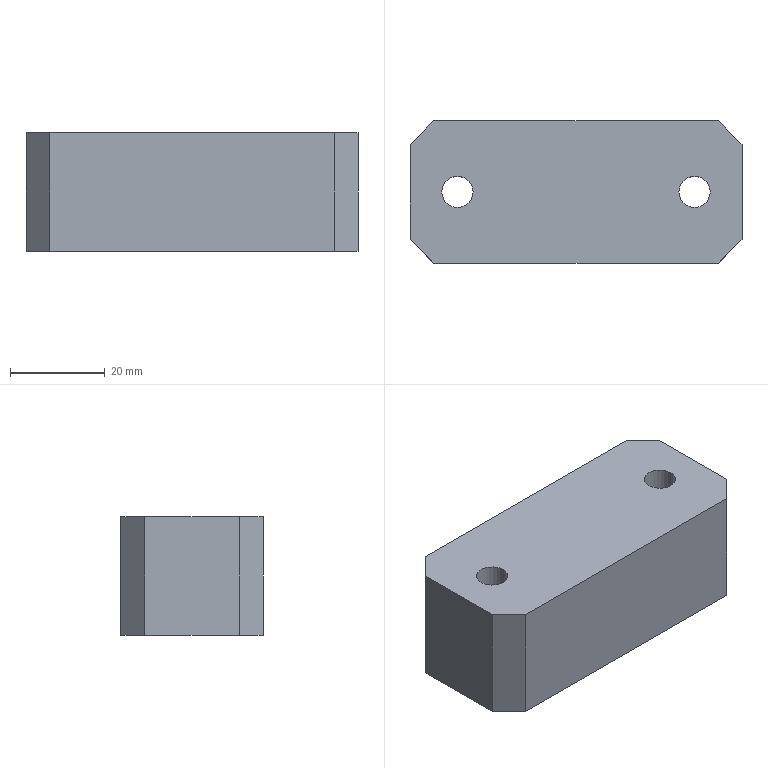Part | STEP file | HXGR200008-05-07 | 1 solid | 38 faces | box 70 x 30 x 25 mm | volume 44261 mm3 | cylinder 16 | plane 14 | cone 8 | commonest cylinder face diameters 6.6 x4 7.9 x4 9 x4 11 x4
STEP:
#1=CARTESIAN_POINT('',(30.5,0.,-5.7));
#2=VERTEX_POINT('',#1);
#3=CARTESIAN_POINT('',(19.5,0.,-5.7));
#4=VERTEX_POINT('',#3);
#5=CARTESIAN_POINT('',(25.,0.,-5.7));
#6=DIRECTION('',(0.,0.,-1.));
#7=DIRECTION('',(-1.,0.,0.));
#8=AXIS2_PLACEMENT_3D('',#5,#6,#7);
#9=CIRCLE('',#8,5.5);
#10=EDGE_CURVE('',#2,#4,#9,.T.);
#11=ORIENTED_EDGE('',*,*,#10,.F.);
#12=CARTESIAN_POINT('',(30.5,0.,-12.5));
#13=VERTEX_POINT('',#12);
#14=CARTESIAN_POINT('',(30.5,0.,-12.5));
#15=DIRECTION('',(0.,0.,-1.));
#16=VECTOR('',#15,1000.);
#17=LINE('',#14,#16);
#18=EDGE_CURVE('',#2,#13,#17,.T.);
#19=ORIENTED_EDGE('',*,*,#18,.T.);
#20=CARTESIAN_POINT('',(19.5,0.,-12.5));
#21=VERTEX_POINT('',#20);
#22=CARTESIAN_POINT('',(25.,0.,-12.5));
#23=DIRECTION('',(0.,0.,-1.));
#24=DIRECTION('',(-1.,0.,0.));
#25=AXIS2_PLACEMENT_3D('',#22,#23,#24);
#26=CIRCLE('',#25,5.5);
#27=EDGE_CURVE('',#13,#21,#26,.T.);
#28=ORIENTED_EDGE('',*,*,#27,.T.);
#29=CARTESIAN_POINT('',(19.5,0.,-12.5));
#30=DIRECTION('',(0.,0.,-1.));
#31=VECTOR('',#30,1000.);
#32=LINE('',#29,#31);
#33=EDGE_CURVE('',#4,#21,#32,.T.);
#34=ORIENTED_EDGE('',*,*,#33,.F.);
#35=EDGE_LOOP('',(#11,#19,#28,#34));
#36=FACE_OUTER_BOUND('',#35,.T.);
#37=CARTESIAN_POINT('',(25.,0.,-12.5));
#38=DIRECTION('',(0.,0.,-1.));
#39=DIRECTION('',(-1.,0.,0.));
#40=AXIS2_PLACEMENT_3D('',#37,#38,#39);
#41=CYLINDRICAL_SURFACE('',#40,5.5);
#42=ADVANCED_FACE('',(#36),#41,.F.);
#43=CARTESIAN_POINT('',(28.3,0.,12.5));
#44=VERTEX_POINT('',#43);
#45=CARTESIAN_POINT('',(21.7,0.,12.5));
#46=VERTEX_POINT('',#45);
#47=CARTESIAN_POINT('',(25.,0.,12.5));
#48=DIRECTION('',(0.,0.,-1.));
#49=DIRECTION('',(-1.,0.,0.));
#50=AXIS2_PLACEMENT_3D('',#47,#48,#49);
#51=CIRCLE('',#50,3.3);
#52=EDGE_CURVE('',#44,#46,#51,.T.);
#53=ORIENTED_EDGE('',*,*,#52,.F.);
#54=CARTESIAN_POINT('',(28.3,0.,-5.7));
#55=VERTEX_POINT('',#54);
#56=CARTESIAN_POINT('',(28.3,0.,-12.5));
#57=DIRECTION('',(0.,0.,-1.));
#58=VECTOR('',#57,1000.);
#59=LINE('',#56,#58);
#60=EDGE_CURVE('',#44,#55,#59,.T.);
#61=ORIENTED_EDGE('',*,*,#60,.T.);
#62=CARTESIAN_POINT('',(21.7,0.,-5.7));
#63=VERTEX_POINT('',#62);
#64=CARTESIAN_POINT('',(25.,0.,-5.7));
#65=DIRECTION('',(0.,0.,-1.));
#66=DIRECTION('',(-1.,0.,0.));
#67=AXIS2_PLACEMENT_3D('',#64,#65,#66);
#68=CIRCLE('',#67,3.3);
#69=EDGE_CURVE('',#55,#63,#68,.T.);
#70=ORIENTED_EDGE('',*,*,#69,.T.);
#71=CARTESIAN_POINT('',(21.7,0.,-12.5));
#72=DIRECTION('',(0.,0.,-1.));
#73=VECTOR('',#72,1000.);
#74=LINE('',#71,#73);
#75=EDGE_CURVE('',#46,#63,#74,.T.);
#76=ORIENTED_EDGE('',*,*,#75,.F.);
#77=EDGE_LOOP('',(#53,#61,#70,#76));
#78=FACE_OUTER_BOUND('',#77,.T.);
#79=CARTESIAN_POINT('',(25.,0.,-12.5));
#80=DIRECTION('',(0.,0.,-1.));
#81=DIRECTION('',(-1.,0.,0.));
#82=AXIS2_PLACEMENT_3D('',#79,#80,#81);
#83=CYLINDRICAL_SURFACE('',#82,3.3);
#84=ADVANCED_FACE('',(#78),#83,.F.);
#85=CARTESIAN_POINT('',(-19.5,0.,-5.7));
#86=VERTEX_POINT('',#85);
#87=CARTESIAN_POINT('',(-30.5,0.,-5.7));
#88=VERTEX_POINT('',#87);
#89=CARTESIAN_POINT('',(-25.,0.,-5.7));
#90=DIRECTION('',(0.,0.,-1.));
#91=DIRECTION('',(-1.,0.,0.));
#92=AXIS2_PLACEMENT_3D('',#89,#90,#91);
#93=CIRCLE('',#92,5.5);
#94=EDGE_CURVE('',#86,#88,#93,.T.);
#95=ORIENTED_EDGE('',*,*,#94,.F.);
#96=CARTESIAN_POINT('',(-19.5,0.,-12.5));
#97=VERTEX_POINT('',#96);
#98=CARTESIAN_POINT('',(-19.5,0.,-12.5));
#99=DIRECTION('',(0.,0.,-1.));
#100=VECTOR('',#99,1000.);
#101=LINE('',#98,#100);
#102=EDGE_CURVE('',#86,#97,#101,.T.);
#103=ORIENTED_EDGE('',*,*,#102,.T.);
#104=CARTESIAN_POINT('',(-30.5,0.,-12.5));
#105=VERTEX_POINT('',#104);
#106=CARTESIAN_POINT('',(-25.,0.,-12.5));
#107=DIRECTION('',(0.,0.,-1.));
#108=DIRECTION('',(-1.,0.,0.));
#109=AXIS2_PLACEMENT_3D('',#106,#107,#108);
#110=CIRCLE('',#109,5.5);
#111=EDGE_CURVE('',#97,#105,#110,.T.);
#112=ORIENTED_EDGE('',*,*,#111,.T.);
#113=CARTESIAN_POINT('',(-30.5,0.,-12.5));
#114=DIRECTION('',(0.,0.,-1.));
#115=VECTOR('',#114,1000.);
#116=LINE('',#113,#115);
#117=EDGE_CURVE('',#88,#105,#116,.T.);
#118=ORIENTED_EDGE('',*,*,#117,.F.);
#119=EDGE_LOOP('',(#95,#103,#112,#118));
#120=FACE_OUTER_BOUND('',#119,.T.);
#121=CARTESIAN_POINT('',(-25.,0.,-12.5));
#122=DIRECTION('',(0.,0.,-1.));
#123=DIRECTION('',(-1.,0.,0.));
#124=AXIS2_PLACEMENT_3D('',#121,#122,#123);
#125=CYLINDRICAL_SURFACE('',#124,5.5);
#126=ADVANCED_FACE('',(#120),#125,.F.);
#127=CARTESIAN_POINT('',(-21.7,0.,12.5));
#128=VERTEX_POINT('',#127);
#129=CARTESIAN_POINT('',(-28.3,0.,12.5));
#130=VERTEX_POINT('',#129);
#131=CARTESIAN_POINT('',(-25.,0.,12.5));
#132=DIRECTION('',(0.,0.,-1.));
#133=DIRECTION('',(-1.,0.,0.));
#134=AXIS2_PLACEMENT_3D('',#131,#132,#133);
#135=CIRCLE('',#134,3.3);
#136=EDGE_CURVE('',#128,#130,#135,.T.);
#137=ORIENTED_EDGE('',*,*,#136,.F.);
#138=CARTESIAN_POINT('',(-21.7,0.,-5.7));
#139=VERTEX_POINT('',#138);
#140=CARTESIAN_POINT('',(-21.7,0.,-12.5));
#141=DIRECTION('',(0.,0.,-1.));
#142=VECTOR('',#141,1000.);
#143=LINE('',#140,#142);
#144=EDGE_CURVE('',#128,#139,#143,.T.);
#145=ORIENTED_EDGE('',*,*,#144,.T.);
#146=CARTESIAN_POINT('',(-28.3,0.,-5.7));
#147=VERTEX_POINT('',#146);
#148=CARTESIAN_POINT('',(-25.,0.,-5.7));
#149=DIRECTION('',(0.,0.,-1.));
#150=DIRECTION('',(-1.,0.,0.));
#151=AXIS2_PLACEMENT_3D('',#148,#149,#150);
#152=CIRCLE('',#151,3.3);
#153=EDGE_CURVE('',#139,#147,#152,.T.);
#154=ORIENTED_EDGE('',*,*,#153,.T.);
#155=CARTESIAN_POINT('',(-28.3,0.,-12.5));
#156=DIRECTION('',(0.,0.,-1.));
#157=VECTOR('',#156,1000.);
#158=LINE('',#155,#157);
#159=EDGE_CURVE('',#130,#147,#158,.T.);
#160=ORIENTED_EDGE('',*,*,#159,.F.);
#161=EDGE_LOOP('',(#137,#145,#154,#160));
#162=FACE_OUTER_BOUND('',#161,.T.);
#163=CARTESIAN_POINT('',(-25.,0.,-12.5));
#164=DIRECTION('',(0.,0.,-1.));
#165=DIRECTION('',(-1.,0.,0.));
#166=AXIS2_PLACEMENT_3D('',#163,#164,#165);
#167=CYLINDRICAL_SURFACE('',#166,3.3);
#168=ADVANCED_FACE('',(#162),#167,.F.);
#169=CARTESIAN_POINT('',(14.633,-5.,-5.1));
#170=VERTEX_POINT('',#169);
#171=CARTESIAN_POINT('',(5.367,-5.,-5.1));
#172=VERTEX_POINT('',#171);
#173=CARTESIAN_POINT('',(10.,-5.,-5.1));
#174=DIRECTION('',(0.,0.,-1.));
#175=DIRECTION('',(-1.,0.,0.));
#176=AXIS2_PLACEMENT_3D('',#173,#174,#175);
#177=CIRCLE('',#176,4.633);
#178=EDGE_CURVE('',#170,#172,#177,.T.);
#179=ORIENTED_EDGE('',*,*,#178,.F.);
#180=CARTESIAN_POINT('',(14.864,-5.,-12.5));
#181=VERTEX_POINT('',#180);
#182=CARTESIAN_POINT('',(14.864,-5.,-12.5));
#183=DIRECTION('',(0.0312,0.,-0.9995));
#184=VECTOR('',#183,1000.);
#185=LINE('',#182,#184);
#186=EDGE_CURVE('',#170,#181,#185,.T.);
#187=ORIENTED_EDGE('',*,*,#186,.T.);
#188=CARTESIAN_POINT('',(5.136,-5.,-12.5));
#189=VERTEX_POINT('',#188);
#190=CARTESIAN_POINT('',(10.,-5.,-12.5));
#191=DIRECTION('',(0.,0.,-1.));
#192=DIRECTION('',(-1.,0.,0.));
#193=AXIS2_PLACEMENT_3D('',#190,#191,#192);
#194=CIRCLE('',#193,4.864);
#195=EDGE_CURVE('',#181,#189,#194,.T.);
#196=ORIENTED_EDGE('',*,*,#195,.T.);
#197=CARTESIAN_POINT('',(5.136,-5.,-12.5));
#198=DIRECTION('',(-0.0312,0.,-0.9995));
#199=VECTOR('',#198,1000.);
#200=LINE('',#197,#199);
#201=EDGE_CURVE('',#172,#189,#200,.T.);
#202=ORIENTED_EDGE('',*,*,#201,.F.);
#203=EDGE_LOOP('',(#179,#187,#196,#202));
#204=FACE_OUTER_BOUND('',#203,.T.);
#205=CARTESIAN_POINT('',(10.,-5.,-12.5));
#206=DIRECTION('',(0.,0.,-1.));
#207=DIRECTION('',(-1.,0.,0.));
#208=AXIS2_PLACEMENT_3D('',#205,#206,#207);
#209=CONICAL_SURFACE('',#208,4.864,0.03121);
#210=ADVANCED_FACE('',(#204),#209,.F.);
#211=CARTESIAN_POINT('',(13.95,-5.,-2.156));
#212=VERTEX_POINT('',#211);
#213=CARTESIAN_POINT('',(10.,-8.95,-4.5));
#214=VERTEX_POINT('',#213);
#215=CARTESIAN_POINT('',(13.95,-5.,-2.156));
#216=CARTESIAN_POINT('',(13.95,-5.141,-2.156));
#217=CARTESIAN_POINT('',(13.943,-5.279,-2.17));
#218=CARTESIAN_POINT('',(13.913,-5.554,-2.222));
#219=CARTESIAN_POINT('',(13.892,-5.69,-2.26));
#220=CARTESIAN_POINT('',(13.809,-6.078,-2.398));
#221=CARTESIAN_POINT('',(13.731,-6.321,-2.522));
#222=CARTESIAN_POINT('',(13.537,-6.776,-2.787));
#223=CARTESIAN_POINT('',(13.422,-6.987,-2.929));
#224=CARTESIAN_POINT('',(13.157,-7.386,-3.213));
#225=CARTESIAN_POINT('',(13.005,-7.576,-3.357));
#226=CARTESIAN_POINT('',(12.665,-7.926,-3.633));
#227=CARTESIAN_POINT('',(12.479,-8.086,-3.763));
#228=CARTESIAN_POINT('',(12.07,-8.374,-4.003));
#229=CARTESIAN_POINT('',(11.845,-8.503,-4.113));
#230=CARTESIAN_POINT('',(11.358,-8.719,-4.298));
#231=CARTESIAN_POINT('',(11.102,-8.803,-4.372));
#232=CARTESIAN_POINT('',(10.695,-8.891,-4.448));
#233=CARTESIAN_POINT('',(10.556,-8.913,-4.468));
#234=CARTESIAN_POINT('',(10.279,-8.943,-4.494));
#235=CARTESIAN_POINT('',(10.14,-8.95,-4.5));
#236=CARTESIAN_POINT('',(10.,-8.95,-4.5));
#237=B_SPLINE_CURVE_WITH_KNOTS('',3,(#215,#216,#217,#218,#219,#220,#221,#222,#223,#224,#225,#226,#227,#228,#229,#230,#231,#232,#233,#234,#235,#236),.UNSPECIFIED.,.F.,.F.,(4,2,2,2,2,2,2,2,2,2,4),(0.0134,0.01381,0.01423,0.01506,0.0159,0.01673,0.01757,0.0184,0.01924,0.01965,0.02007),.UNSPECIFIED.);
#238=EDGE_CURVE('',#212,#214,#237,.T.);
#239=ORIENTED_EDGE('',*,*,#238,.F.);
#240=CARTESIAN_POINT('',(13.95,-5.,-5.1));
#241=VERTEX_POINT('',#240);
#242=CARTESIAN_POINT('',(13.95,-5.,-12.5));
#243=DIRECTION('',(0.,0.,-1.));
#244=VECTOR('',#243,1000.);
#245=LINE('',#242,#244);
#246=EDGE_CURVE('',#212,#241,#245,.T.);
#247=ORIENTED_EDGE('',*,*,#246,.T.);
#248=CARTESIAN_POINT('',(6.05,-5.,-5.1));
#249=VERTEX_POINT('',#248);
#250=CARTESIAN_POINT('',(10.,-5.,-5.1));
#251=DIRECTION('',(0.,0.,-1.));
#252=DIRECTION('',(-1.,0.,0.));
#253=AXIS2_PLACEMENT_3D('',#250,#251,#252);
#254=CIRCLE('',#253,3.95);
#255=EDGE_CURVE('',#241,#249,#254,.T.);
#256=ORIENTED_EDGE('',*,*,#255,.T.);
#257=CARTESIAN_POINT('',(6.05,-5.,-2.156));
#258=VERTEX_POINT('',#257);
#259=CARTESIAN_POINT('',(6.05,-5.,-12.5));
#260=DIRECTION('',(0.,0.,-1.));
#261=VECTOR('',#260,1000.);
#262=LINE('',#259,#261);
#263=EDGE_CURVE('',#258,#249,#262,.T.);
#264=ORIENTED_EDGE('',*,*,#263,.F.);
#265=CARTESIAN_POINT('',(10.,-8.95,-4.5));
#266=CARTESIAN_POINT('',(9.722,-8.95,-4.5));
#267=CARTESIAN_POINT('',(9.439,-8.92,-4.473));
#268=CARTESIAN_POINT('',(8.902,-8.804,-4.372));
#269=CARTESIAN_POINT('',(8.641,-8.718,-4.298));
#270=CARTESIAN_POINT('',(8.158,-8.504,-4.114));
#271=CARTESIAN_POINT('',(7.933,-8.376,-4.004));
#272=CARTESIAN_POINT('',(7.518,-8.083,-3.761));
#273=CARTESIAN_POINT('',(7.332,-7.923,-3.63));
#274=CARTESIAN_POINT('',(6.995,-7.575,-3.357));
#275=CARTESIAN_POINT('',(6.844,-7.387,-3.213));
#276=CARTESIAN_POINT('',(6.577,-6.985,-2.927));
#277=CARTESIAN_POINT('',(6.462,-6.774,-2.786));
#278=CARTESIAN_POINT('',(6.319,-6.437,-2.589));
#279=CARTESIAN_POINT('',(6.275,-6.321,-2.526));
#280=CARTESIAN_POINT('',(6.198,-6.079,-2.409));
#281=CARTESIAN_POINT('',(6.164,-5.953,-2.354));
#282=CARTESIAN_POINT('',(6.109,-5.692,-2.261));
#283=CARTESIAN_POINT('',(6.087,-5.559,-2.223));
#284=CARTESIAN_POINT('',(6.058,-5.284,-2.17));
#285=CARTESIAN_POINT('',(6.05,-5.141,-2.156));
#286=CARTESIAN_POINT('',(6.05,-5.,-2.156));
#287=B_SPLINE_CURVE_WITH_KNOTS('',3,(#265,#266,#267,#268,#269,#270,#271,#272,#273,#274,#275,#276,#277,#278,#279,#280,#281,#282,#283,#284,#285,#286),.UNSPECIFIED.,.F.,.F.,(4,2,2,2,2,2,2,2,2,2,4),(0.02007,0.0209,0.02174,0.02257,0.0234,0.02423,0.02506,0.02548,0.02589,0.02631,0.02673),.UNSPECIFIED.);
#288=EDGE_CURVE('',#214,#258,#287,.T.);
#289=ORIENTED_EDGE('',*,*,#288,.F.);
#290=EDGE_LOOP('',(#239,#247,#256,#264,#289));
#291=FACE_OUTER_BOUND('',#290,.T.);
#292=CARTESIAN_POINT('',(10.,-5.,-12.5));
#293=DIRECTION('',(0.,0.,-1.));
#294=DIRECTION('',(-1.,0.,0.));
#295=AXIS2_PLACEMENT_3D('',#292,#293,#294);
#296=CYLINDRICAL_SURFACE('',#295,3.95);
#297=ADVANCED_FACE('',(#291),#296,.F.);
#298=CARTESIAN_POINT('',(-5.367,-5.,-5.1));
#299=VERTEX_POINT('',#298);
#300=CARTESIAN_POINT('',(-14.633,-5.,-5.1));
#301=VERTEX_POINT('',#300);
#302=CARTESIAN_POINT('',(-10.,-5.,-5.1));
#303=DIRECTION('',(0.,0.,-1.));
#304=DIRECTION('',(-1.,0.,0.));
#305=AXIS2_PLACEMENT_3D('',#302,#303,#304);
#306=CIRCLE('',#305,4.633);
#307=EDGE_CURVE('',#299,#301,#306,.T.);
#308=ORIENTED_EDGE('',*,*,#307,.F.);
#309=CARTESIAN_POINT('',(-5.136,-5.,-12.5));
#310=VERTEX_POINT('',#309);
#311=CARTESIAN_POINT('',(-5.136,-5.,-12.5));
#312=DIRECTION('',(0.0312,0.,-0.9995));
#313=VECTOR('',#312,1000.);
#314=LINE('',#311,#313);
#315=EDGE_CURVE('',#299,#310,#314,.T.);
#316=ORIENTED_EDGE('',*,*,#315,.T.);
#317=CARTESIAN_POINT('',(-14.864,-5.,-12.5));
#318=VERTEX_POINT('',#317);
#319=CARTESIAN_POINT('',(-10.,-5.,-12.5));
#320=DIRECTION('',(0.,0.,-1.));
#321=DIRECTION('',(-1.,0.,0.));
#322=AXIS2_PLACEMENT_3D('',#319,#320,#321);
#323=CIRCLE('',#322,4.864);
#324=EDGE_CURVE('',#310,#318,#323,.T.);
#325=ORIENTED_EDGE('',*,*,#324,.T.);
#326=CARTESIAN_POINT('',(-14.864,-5.,-12.5));
#327=DIRECTION('',(-0.0312,0.,-0.9995));
#328=VECTOR('',#327,1000.);
#329=LINE('',#326,#328);
#330=EDGE_CURVE('',#301,#318,#329,.T.);
#331=ORIENTED_EDGE('',*,*,#330,.F.);
#332=EDGE_LOOP('',(#308,#316,#325,#331));
#333=FACE_OUTER_BOUND('',#332,.T.);
#334=CARTESIAN_POINT('',(-10.,-5.,-12.5));
#335=DIRECTION('',(0.,0.,-1.));
#336=DIRECTION('',(-1.,0.,0.));
#337=AXIS2_PLACEMENT_3D('',#334,#335,#336);
#338=CONICAL_SURFACE('',#337,4.864,0.03121);
#339=ADVANCED_FACE('',(#333),#338,.F.);
#340=CARTESIAN_POINT('',(-6.05,-5.,-2.156));
#341=VERTEX_POINT('',#340);
#342=CARTESIAN_POINT('',(-10.,-8.95,-4.5));
#343=VERTEX_POINT('',#342);
#344=CARTESIAN_POINT('',(-6.05,-5.,-2.156));
#345=CARTESIAN_POINT('',(-6.05,-5.141,-2.156));
#346=CARTESIAN_POINT('',(-6.057,-5.279,-2.17));
#347=CARTESIAN_POINT('',(-6.087,-5.554,-2.222));
#348=CARTESIAN_POINT('',(-6.108,-5.69,-2.26));
#349=CARTESIAN_POINT('',(-6.191,-6.078,-2.398));
#350=CARTESIAN_POINT('',(-6.269,-6.321,-2.522));
#351=CARTESIAN_POINT('',(-6.463,-6.776,-2.787));
#352=CARTESIAN_POINT('',(-6.578,-6.987,-2.929));
#353=CARTESIAN_POINT('',(-6.843,-7.386,-3.213));
#354=CARTESIAN_POINT('',(-6.995,-7.576,-3.357));
#355=CARTESIAN_POINT('',(-7.335,-7.926,-3.633));
#356=CARTESIAN_POINT('',(-7.521,-8.086,-3.763));
#357=CARTESIAN_POINT('',(-7.93,-8.374,-4.003));
#358=CARTESIAN_POINT('',(-8.155,-8.503,-4.113));
#359=CARTESIAN_POINT('',(-8.642,-8.719,-4.298));
#360=CARTESIAN_POINT('',(-8.898,-8.803,-4.372));
#361=CARTESIAN_POINT('',(-9.305,-8.891,-4.448));
#362=CARTESIAN_POINT('',(-9.444,-8.913,-4.468));
#363=CARTESIAN_POINT('',(-9.721,-8.943,-4.494));
#364=CARTESIAN_POINT('',(-9.86,-8.95,-4.5));
#365=CARTESIAN_POINT('',(-10.,-8.95,-4.5));
#366=B_SPLINE_CURVE_WITH_KNOTS('',3,(#344,#345,#346,#347,#348,#349,#350,#351,#352,#353,#354,#355,#356,#357,#358,#359,#360,#361,#362,#363,#364,#365),.UNSPECIFIED.,.F.,.F.,(4,2,2,2,2,2,2,2,2,2,4),(0.0134,0.01381,0.01423,0.01506,0.0159,0.01673,0.01757,0.0184,0.01924,0.01965,0.02007),.UNSPECIFIED.);
#367=EDGE_CURVE('',#341,#343,#366,.T.);
#368=ORIENTED_EDGE('',*,*,#367,.F.);
#369=CARTESIAN_POINT('',(-6.05,-5.,-5.1));
#370=VERTEX_POINT('',#369);
#371=CARTESIAN_POINT('',(-6.05,-5.,-12.5));
#372=DIRECTION('',(0.,0.,-1.));
#373=VECTOR('',#372,1000.);
#374=LINE('',#371,#373);
#375=EDGE_CURVE('',#341,#370,#374,.T.);
#376=ORIENTED_EDGE('',*,*,#375,.T.);
#377=CARTESIAN_POINT('',(-13.95,-5.,-5.1));
#378=VERTEX_POINT('',#377);
#379=CARTESIAN_POINT('',(-10.,-5.,-5.1));
#380=DIRECTION('',(0.,0.,-1.));
#381=DIRECTION('',(-1.,0.,0.));
#382=AXIS2_PLACEMENT_3D('',#379,#380,#381);
#383=CIRCLE('',#382,3.95);
#384=EDGE_CURVE('',#370,#378,#383,.T.);
#385=ORIENTED_EDGE('',*,*,#384,.T.);
#386=CARTESIAN_POINT('',(-13.95,-5.,-2.156));
#387=VERTEX_POINT('',#386);
#388=CARTESIAN_POINT('',(-13.95,-5.,-12.5));
#389=DIRECTION('',(0.,0.,-1.));
#390=VECTOR('',#389,1000.);
#391=LINE('',#388,#390);
#392=EDGE_CURVE('',#387,#378,#391,.T.);
#393=ORIENTED_EDGE('',*,*,#392,.F.);
#394=CARTESIAN_POINT('',(-10.,-8.95,-4.5));
#395=CARTESIAN_POINT('',(-10.278,-8.95,-4.5));
#396=CARTESIAN_POINT('',(-10.561,-8.92,-4.473));
#397=CARTESIAN_POINT('',(-11.098,-8.804,-4.372));
#398=CARTESIAN_POINT('',(-11.359,-8.718,-4.298));
#399=CARTESIAN_POINT('',(-11.842,-8.504,-4.114));
#400=CARTESIAN_POINT('',(-12.067,-8.376,-4.004));
#401=CARTESIAN_POINT('',(-12.482,-8.083,-3.761));
#402=CARTESIAN_POINT('',(-12.668,-7.923,-3.63));
#403=CARTESIAN_POINT('',(-13.005,-7.575,-3.357));
#404=CARTESIAN_POINT('',(-13.156,-7.387,-3.213));
#405=CARTESIAN_POINT('',(-13.423,-6.985,-2.927));
#406=CARTESIAN_POINT('',(-13.538,-6.774,-2.786));
#407=CARTESIAN_POINT('',(-13.681,-6.437,-2.589));
#408=CARTESIAN_POINT('',(-13.725,-6.321,-2.526));
#409=CARTESIAN_POINT('',(-13.802,-6.079,-2.409));
#410=CARTESIAN_POINT('',(-13.836,-5.953,-2.354));
#411=CARTESIAN_POINT('',(-13.891,-5.692,-2.261));
#412=CARTESIAN_POINT('',(-13.913,-5.559,-2.223));
#413=CARTESIAN_POINT('',(-13.942,-5.284,-2.17));
#414=CARTESIAN_POINT('',(-13.95,-5.141,-2.156));
#415=CARTESIAN_POINT('',(-13.95,-5.,-2.156));
#416=B_SPLINE_CURVE_WITH_KNOTS('',3,(#394,#395,#396,#397,#398,#399,#400,#401,#402,#403,#404,#405,#406,#407,#408,#409,#410,#411,#412,#413,#414,#415),.UNSPECIFIED.,.F.,.F.,(4,2,2,2,2,2,2,2,2,2,4),(0.02007,0.0209,0.02174,0.02257,0.0234,0.02423,0.02506,0.02548,0.02589,0.02631,0.02673),.UNSPECIFIED.);
#417=EDGE_CURVE('',#343,#387,#416,.T.);
#418=ORIENTED_EDGE('',*,*,#417,.F.);
#419=EDGE_LOOP('',(#368,#376,#385,#393,#418));
#420=FACE_OUTER_BOUND('',#419,.T.);
#421=CARTESIAN_POINT('',(-10.,-5.,-12.5));
#422=DIRECTION('',(0.,0.,-1.));
#423=DIRECTION('',(-1.,0.,0.));
#424=AXIS2_PLACEMENT_3D('',#421,#422,#423);
#425=CYLINDRICAL_SURFACE('',#424,3.95);
#426=ADVANCED_FACE('',(#420),#425,.F.);
#427=CARTESIAN_POINT('',(10.,-10.,-4.5));
#428=VERTEX_POINT('',#427);
#429=CARTESIAN_POINT('',(10.,-10.,4.5));
#430=VERTEX_POINT('',#429);
#431=CARTESIAN_POINT('',(10.,-10.,0.));
#432=DIRECTION('',(0.,1.,0.));
#433=DIRECTION('',(0.,0.,1.));
#434=AXIS2_PLACEMENT_3D('',#431,#432,#433);
#435=CIRCLE('',#434,4.5);
#436=EDGE_CURVE('',#428,#430,#435,.T.);
#437=ORIENTED_EDGE('',*,*,#436,.F.);
#438=CARTESIAN_POINT('',(10.,15.,-4.5));
#439=DIRECTION('',(0.,1.,0.));
#440=VECTOR('',#439,1000.);
#441=LINE('',#438,#440);
#442=EDGE_CURVE('',#428,#214,#441,.T.);
#443=ORIENTED_EDGE('',*,*,#442,.T.);
#444=ORIENTED_EDGE('',*,*,#288,.T.);
#445=CARTESIAN_POINT('',(10.,-1.05,-4.5));
#446=VERTEX_POINT('',#445);
#447=CARTESIAN_POINT('',(6.05,-5.,-2.156));
#448=CARTESIAN_POINT('',(6.05,-4.858,-2.156));
#449=CARTESIAN_POINT('',(6.058,-4.719,-2.17));
#450=CARTESIAN_POINT('',(6.087,-4.446,-2.222));
#451=CARTESIAN_POINT('',(6.108,-4.311,-2.26));
#452=CARTESIAN_POINT('',(6.191,-3.92,-2.399));
#453=CARTESIAN_POINT('',(6.269,-3.681,-2.521));
#454=CARTESIAN_POINT('',(6.462,-3.226,-2.786));
#455=CARTESIAN_POINT('',(6.578,-3.012,-2.929));
#456=CARTESIAN_POINT('',(6.843,-2.614,-3.213));
#457=CARTESIAN_POINT('',(6.993,-2.427,-3.355));
#458=CARTESIAN_POINT('',(7.332,-2.077,-3.63));
#459=CARTESIAN_POINT('',(7.522,-1.914,-3.764));
#460=CARTESIAN_POINT('',(7.933,-1.625,-4.004));
#461=CARTESIAN_POINT('',(8.157,-1.496,-4.114));
#462=CARTESIAN_POINT('',(8.644,-1.28,-4.299));
#463=CARTESIAN_POINT('',(8.9,-1.196,-4.372));
#464=CARTESIAN_POINT('',(9.305,-1.109,-4.448));
#465=CARTESIAN_POINT('',(9.444,-1.087,-4.468));
#466=CARTESIAN_POINT('',(9.722,-1.057,-4.494));
#467=CARTESIAN_POINT('',(9.861,-1.05,-4.5));
#468=CARTESIAN_POINT('',(10.,-1.05,-4.5));
#469=B_SPLINE_CURVE_WITH_KNOTS('',3,(#447,#448,#449,#450,#451,#452,#453,#454,#455,#456,#457,#458,#459,#460,#461,#462,#463,#464,#465,#466,#467,#468),.UNSPECIFIED.,.F.,.F.,(4,2,2,2,2,2,2,2,2,2,4),(0.,0.0004189,0.0008378,0.001676,0.002513,0.003351,0.004189,0.005027,0.005865,0.006283,0.006702),.UNSPECIFIED.);
#470=EDGE_CURVE('',#258,#446,#469,.T.);
#471=ORIENTED_EDGE('',*,*,#470,.T.);
#472=CARTESIAN_POINT('',(10.,15.,-4.5));
#473=VERTEX_POINT('',#472);
#474=CARTESIAN_POINT('',(10.,15.,-4.5));
#475=DIRECTION('',(0.,1.,0.));
#476=VECTOR('',#475,1000.);
#477=LINE('',#474,#476);
#478=EDGE_CURVE('',#446,#473,#477,.T.);
#479=ORIENTED_EDGE('',*,*,#478,.T.);
#480=CARTESIAN_POINT('',(10.,15.,4.5));
#481=VERTEX_POINT('',#480);
#482=CARTESIAN_POINT('',(10.,15.,0.));
#483=DIRECTION('',(0.,1.,0.));
#484=DIRECTION('',(0.,0.,1.));
#485=AXIS2_PLACEMENT_3D('',#482,#483,#484);
#486=CIRCLE('',#485,4.5);
#487=EDGE_CURVE('',#473,#481,#486,.T.);
#488=ORIENTED_EDGE('',*,*,#487,.T.);
#489=CARTESIAN_POINT('',(10.,15.,4.5));
#490=DIRECTION('',(0.,1.,0.));
#491=VECTOR('',#490,1000.);
#492=LINE('',#489,#491);
#493=EDGE_CURVE('',#430,#481,#492,.T.);
#494=ORIENTED_EDGE('',*,*,#493,.F.);
#495=EDGE_LOOP('',(#437,#443,#444,#471,#479,#488,#494));
#496=FACE_OUTER_BOUND('',#495,.T.);
#497=CARTESIAN_POINT('',(10.,15.,0.));
#498=DIRECTION('',(0.,1.,0.));
#499=DIRECTION('',(0.,0.,1.));
#500=AXIS2_PLACEMENT_3D('',#497,#498,#499);
#501=CYLINDRICAL_SURFACE('',#500,4.5);
#502=ADVANCED_FACE('',(#496),#501,.F.);
#503=CARTESIAN_POINT('',(10.,-12.704,0.));
#504=VERTEX_POINT('',#503);
#505=CARTESIAN_POINT('',(10.,-10.,4.5));
#506=DIRECTION('',(0.,0.515,0.8572));
#507=VECTOR('',#506,1000.);
#508=LINE('',#505,#507);
#509=EDGE_CURVE('',#504,#430,#508,.T.);
#510=ORIENTED_EDGE('',*,*,#509,.F.);
#511=CARTESIAN_POINT('',(10.,-10.,-4.5));
#512=DIRECTION('',(0.,0.515,-0.8572));
#513=VECTOR('',#512,1000.);
#514=LINE('',#511,#513);
#515=EDGE_CURVE('',#504,#428,#514,.T.);
#516=ORIENTED_EDGE('',*,*,#515,.T.);
#517=ORIENTED_EDGE('',*,*,#436,.T.);
#518=EDGE_LOOP('',(#510,#516,#517));
#519=FACE_OUTER_BOUND('',#518,.T.);
#520=CARTESIAN_POINT('',(10.,-10.,0.));
#521=DIRECTION('',(0.,1.,0.));
#522=DIRECTION('',(0.,0.,1.));
#523=AXIS2_PLACEMENT_3D('',#520,#521,#522);
#524=CONICAL_SURFACE('',#523,4.5,1.03);
#525=ADVANCED_FACE('',(#519),#524,.F.);
#526=CARTESIAN_POINT('',(-10.,-10.,-4.5));
#527=VERTEX_POINT('',#526);
#528=CARTESIAN_POINT('',(-10.,-10.,4.5));
#529=VERTEX_POINT('',#528);
#530=CARTESIAN_POINT('',(-10.,-10.,0.));
#531=DIRECTION('',(0.,1.,0.));
#532=DIRECTION('',(0.,0.,1.));
#533=AXIS2_PLACEMENT_3D('',#530,#531,#532);
#534=CIRCLE('',#533,4.5);
#535=EDGE_CURVE('',#527,#529,#534,.T.);
#536=ORIENTED_EDGE('',*,*,#535,.F.);
#537=CARTESIAN_POINT('',(-10.,15.,-4.5));
#538=DIRECTION('',(0.,1.,0.));
#539=VECTOR('',#538,1000.);
#540=LINE('',#537,#539);
#541=EDGE_CURVE('',#527,#343,#540,.T.);
#542=ORIENTED_EDGE('',*,*,#541,.T.);
#543=ORIENTED_EDGE('',*,*,#417,.T.);
#544=CARTESIAN_POINT('',(-10.,-1.05,-4.5));
#545=VERTEX_POINT('',#544);
#546=CARTESIAN_POINT('',(-13.95,-5.,-2.156));
#547=CARTESIAN_POINT('',(-13.95,-4.858,-2.156));
#548=CARTESIAN_POINT('',(-13.942,-4.719,-2.17));
#549=CARTESIAN_POINT('',(-13.913,-4.446,-2.222));
#550=CARTESIAN_POINT('',(-13.892,-4.311,-2.26));
#551=CARTESIAN_POINT('',(-13.809,-3.92,-2.399));
#552=CARTESIAN_POINT('',(-13.731,-3.681,-2.521));
#553=CARTESIAN_POINT('',(-13.538,-3.226,-2.786));
#554=CARTESIAN_POINT('',(-13.422,-3.012,-2.929));
#555=CARTESIAN_POINT('',(-13.157,-2.614,-3.213));
#556=CARTESIAN_POINT('',(-13.007,-2.427,-3.355));
#557=CARTESIAN_POINT('',(-12.668,-2.077,-3.63));
#558=CARTESIAN_POINT('',(-12.478,-1.914,-3.764));
#559=CARTESIAN_POINT('',(-12.067,-1.625,-4.004));
#560=CARTESIAN_POINT('',(-11.843,-1.496,-4.114));
#561=CARTESIAN_POINT('',(-11.356,-1.28,-4.299));
#562=CARTESIAN_POINT('',(-11.1,-1.196,-4.372));
#563=CARTESIAN_POINT('',(-10.695,-1.109,-4.448));
#564=CARTESIAN_POINT('',(-10.556,-1.087,-4.468));
#565=CARTESIAN_POINT('',(-10.278,-1.057,-4.494));
#566=CARTESIAN_POINT('',(-10.139,-1.05,-4.5));
#567=CARTESIAN_POINT('',(-10.,-1.05,-4.5));
#568=B_SPLINE_CURVE_WITH_KNOTS('',3,(#546,#547,#548,#549,#550,#551,#552,#553,#554,#555,#556,#557,#558,#559,#560,#561,#562,#563,#564,#565,#566,#567),.UNSPECIFIED.,.F.,.F.,(4,2,2,2,2,2,2,2,2,2,4),(0.,0.0004189,0.0008378,0.001676,0.002513,0.003351,0.004189,0.005027,0.005865,0.006283,0.006702),.UNSPECIFIED.);
#569=EDGE_CURVE('',#387,#545,#568,.T.);
#570=ORIENTED_EDGE('',*,*,#569,.T.);
#571=CARTESIAN_POINT('',(-10.,15.,-4.5));
#572=VERTEX_POINT('',#571);
#573=CARTESIAN_POINT('',(-10.,15.,-4.5));
#574=DIRECTION('',(0.,1.,0.));
#575=VECTOR('',#574,1000.);
#576=LINE('',#573,#575);
#577=EDGE_CURVE('',#545,#572,#576,.T.);
#578=ORIENTED_EDGE('',*,*,#577,.T.);
#579=CARTESIAN_POINT('',(-10.,15.,4.5));
#580=VERTEX_POINT('',#579);
#581=CARTESIAN_POINT('',(-10.,15.,0.));
#582=DIRECTION('',(0.,1.,0.));
#583=DIRECTION('',(0.,0.,1.));
#584=AXIS2_PLACEMENT_3D('',#581,#582,#583);
#585=CIRCLE('',#584,4.5);
#586=EDGE_CURVE('',#572,#580,#585,.T.);
#587=ORIENTED_EDGE('',*,*,#586,.T.);
#588=CARTESIAN_POINT('',(-10.,15.,4.5));
#589=DIRECTION('',(0.,1.,0.));
#590=VECTOR('',#589,1000.);
#591=LINE('',#588,#590);
#592=EDGE_CURVE('',#529,#580,#591,.T.);
#593=ORIENTED_EDGE('',*,*,#592,.F.);
#594=EDGE_LOOP('',(#536,#542,#543,#570,#578,#587,#593));
#595=FACE_OUTER_BOUND('',#594,.T.);
#596=CARTESIAN_POINT('',(-10.,15.,0.));
#597=DIRECTION('',(0.,1.,0.));
#598=DIRECTION('',(0.,0.,1.));
#599=AXIS2_PLACEMENT_3D('',#596,#597,#598);
#600=CYLINDRICAL_SURFACE('',#599,4.5);
#601=ADVANCED_FACE('',(#595),#600,.F.);
#602=CARTESIAN_POINT('',(-10.,-12.704,0.));
#603=VERTEX_POINT('',#602);
#604=CARTESIAN_POINT('',(-10.,-10.,4.5));
#605=DIRECTION('',(0.,0.515,0.8572));
#606=VECTOR('',#605,1000.);
#607=LINE('',#604,#606);
#608=EDGE_CURVE('',#603,#529,#607,.T.);
#609=ORIENTED_EDGE('',*,*,#608,.F.);
#610=CARTESIAN_POINT('',(-10.,-10.,-4.5));
#611=DIRECTION('',(0.,0.515,-0.8572));
#612=VECTOR('',#611,1000.);
#613=LINE('',#610,#612);
#614=EDGE_CURVE('',#603,#527,#613,.T.);
#615=ORIENTED_EDGE('',*,*,#614,.T.);
#616=ORIENTED_EDGE('',*,*,#535,.T.);
#617=EDGE_LOOP('',(#609,#615,#616));
#618=FACE_OUTER_BOUND('',#617,.T.);
#619=CARTESIAN_POINT('',(-10.,-10.,0.));
#620=DIRECTION('',(0.,1.,0.));
#621=DIRECTION('',(0.,0.,1.));
#622=AXIS2_PLACEMENT_3D('',#619,#620,#621);
#623=CONICAL_SURFACE('',#622,4.5,1.03);
#624=ADVANCED_FACE('',(#618),#623,.F.);
#625=CARTESIAN_POINT('',(25.,0.,-12.5));
#626=DIRECTION('',(0.,0.,-1.));
#627=DIRECTION('',(-1.,0.,0.));
#628=AXIS2_PLACEMENT_3D('',#625,#626,#627);
#629=CIRCLE('',#628,5.5);
#630=EDGE_CURVE('',#21,#13,#629,.T.);
#631=ORIENTED_EDGE('',*,*,#630,.F.);
#632=ORIENTED_EDGE('',*,*,#27,.F.);
#633=EDGE_LOOP('',(#631,#632));
#634=FACE_BOUND('',#633,.T.);
#635=CARTESIAN_POINT('',(-25.,0.,-12.5));
#636=DIRECTION('',(0.,0.,-1.));
#637=DIRECTION('',(-1.,0.,0.));
#638=AXIS2_PLACEMENT_3D('',#635,#636,#637);
#639=CIRCLE('',#638,5.5);
#640=EDGE_CURVE('',#105,#97,#639,.T.);
#641=ORIENTED_EDGE('',*,*,#640,.F.);
#642=ORIENTED_EDGE('',*,*,#111,.F.);
#643=EDGE_LOOP('',(#641,#642));
#644=FACE_BOUND('',#643,.T.);
#645=CARTESIAN_POINT('',(35.,-10.,-12.5));
#646=VERTEX_POINT('',#645);
#647=CARTESIAN_POINT('',(35.,10.,-12.5));
#648=VERTEX_POINT('',#647);
#649=CARTESIAN_POINT('',(35.,-15.,-12.5));
#650=DIRECTION('',(0.,1.,0.));
#651=VECTOR('',#650,1000.);
#652=LINE('',#649,#651);
#653=EDGE_CURVE('',#646,#648,#652,.T.);
#654=ORIENTED_EDGE('',*,*,#653,.F.);
#655=CARTESIAN_POINT('',(30.,-15.,-12.5));
#656=VERTEX_POINT('',#655);
#657=CARTESIAN_POINT('',(35.,-10.,-12.5));
#658=DIRECTION('',(-0.7071,-0.7071,0.));
#659=VECTOR('',#658,1000.);
#660=LINE('',#657,#659);
#661=EDGE_CURVE('',#646,#656,#660,.T.);
#662=ORIENTED_EDGE('',*,*,#661,.T.);
#663=CARTESIAN_POINT('',(-30.,-15.,-12.5));
#664=VERTEX_POINT('',#663);
#665=CARTESIAN_POINT('',(35.,-15.,-12.5));
#666=DIRECTION('',(1.,0.,0.));
#667=VECTOR('',#666,1000.);
#668=LINE('',#665,#667);
#669=EDGE_CURVE('',#664,#656,#668,.T.);
#670=ORIENTED_EDGE('',*,*,#669,.F.);
#671=CARTESIAN_POINT('',(-35.,-10.,-12.5));
#672=VERTEX_POINT('',#671);
#673=CARTESIAN_POINT('',(-30.,-15.,-12.5));
#674=DIRECTION('',(-0.7071,0.7071,0.));
#675=VECTOR('',#674,1000.);
#676=LINE('',#673,#675);
#677=EDGE_CURVE('',#664,#672,#676,.T.);
#678=ORIENTED_EDGE('',*,*,#677,.T.);
#679=CARTESIAN_POINT('',(-35.,10.,-12.5));
#680=VERTEX_POINT('',#679);
#681=CARTESIAN_POINT('',(-35.,-15.,-12.5));
#682=DIRECTION('',(0.,-1.,0.));
#683=VECTOR('',#682,1000.);
#684=LINE('',#681,#683);
#685=EDGE_CURVE('',#680,#672,#684,.T.);
#686=ORIENTED_EDGE('',*,*,#685,.F.);
#687=CARTESIAN_POINT('',(-30.,15.,-12.5));
#688=VERTEX_POINT('',#687);
#689=CARTESIAN_POINT('',(-35.,10.,-12.5));
#690=DIRECTION('',(0.7071,0.7071,0.));
#691=VECTOR('',#690,1000.);
#692=LINE('',#689,#691);
#693=EDGE_CURVE('',#680,#688,#692,.T.);
#694=ORIENTED_EDGE('',*,*,#693,.T.);
#695=CARTESIAN_POINT('',(30.,15.,-12.5));
#696=VERTEX_POINT('',#695);
#697=CARTESIAN_POINT('',(35.,15.,-12.5));
#698=DIRECTION('',(-1.,0.,0.));
#699=VECTOR('',#698,1000.);
#700=LINE('',#697,#699);
#701=EDGE_CURVE('',#696,#688,#700,.T.);
#702=ORIENTED_EDGE('',*,*,#701,.F.);
#703=CARTESIAN_POINT('',(30.,15.,-12.5));
#704=DIRECTION('',(0.7071,-0.7071,0.));
#705=VECTOR('',#704,1000.);
#706=LINE('',#703,#705);
#707=EDGE_CURVE('',#696,#648,#706,.T.);
#708=ORIENTED_EDGE('',*,*,#707,.T.);
#709=EDGE_LOOP('',(#654,#662,#670,#678,#686,#694,#702,#708));
#710=FACE_OUTER_BOUND('',#709,.T.);
#711=CARTESIAN_POINT('',(-10.,-5.,-12.5));
#712=DIRECTION('',(0.,0.,-1.));
#713=DIRECTION('',(-1.,0.,0.));
#714=AXIS2_PLACEMENT_3D('',#711,#712,#713);
#715=CIRCLE('',#714,4.864);
#716=EDGE_CURVE('',#318,#310,#715,.T.);
#717=ORIENTED_EDGE('',*,*,#716,.F.);
#718=ORIENTED_EDGE('',*,*,#324,.F.);
#719=EDGE_LOOP('',(#717,#718));
#720=FACE_BOUND('',#719,.T.);
#721=CARTESIAN_POINT('',(10.,-5.,-12.5));
#722=DIRECTION('',(0.,0.,-1.));
#723=DIRECTION('',(-1.,0.,0.));
#724=AXIS2_PLACEMENT_3D('',#721,#722,#723);
#725=CIRCLE('',#724,4.864);
#726=EDGE_CURVE('',#189,#181,#725,.T.);
#727=ORIENTED_EDGE('',*,*,#726,.F.);
#728=ORIENTED_EDGE('',*,*,#195,.F.);
#729=EDGE_LOOP('',(#727,#728));
#730=FACE_BOUND('',#729,.T.);
#731=CARTESIAN_POINT('',(0.,0.,-12.5));
#732=DIRECTION('',(0.,0.,1.));
#733=DIRECTION('',(1.,0.,0.));
#734=AXIS2_PLACEMENT_3D('',#731,#732,#733);
#735=PLANE('',#734);
#736=ADVANCED_FACE('',(#634,#644,#710,#720,#730),#735,.F.);
#737=ORIENTED_EDGE('',*,*,#685,.T.);
#738=CARTESIAN_POINT('',(-35.,-10.,12.5));
#739=VERTEX_POINT('',#738);
#740=CARTESIAN_POINT('',(-35.,-10.,12.5));
#741=DIRECTION('',(0.,0.,1.));
#742=VECTOR('',#741,1000.);
#743=LINE('',#740,#742);
#744=EDGE_CURVE('',#672,#739,#743,.T.);
#745=ORIENTED_EDGE('',*,*,#744,.T.);
#746=CARTESIAN_POINT('',(-35.,10.,12.5));
#747=VERTEX_POINT('',#746);
#748=CARTESIAN_POINT('',(-35.,-15.,12.5));
#749=DIRECTION('',(0.,-1.,0.));
#750=VECTOR('',#749,1000.);
#751=LINE('',#748,#750);
#752=EDGE_CURVE('',#747,#739,#751,.T.);
#753=ORIENTED_EDGE('',*,*,#752,.F.);
#754=CARTESIAN_POINT('',(-35.,10.,12.5));
#755=DIRECTION('',(0.,0.,-1.));
#756=VECTOR('',#755,1000.);
#757=LINE('',#754,#756);
#758=EDGE_CURVE('',#747,#680,#757,.T.);
#759=ORIENTED_EDGE('',*,*,#758,.T.);
#760=EDGE_LOOP('',(#737,#745,#753,#759));
#761=FACE_OUTER_BOUND('',#760,.T.);
#762=CARTESIAN_POINT('',(-35.,-15.,12.5));
#763=DIRECTION('',(1.,0.,0.));
#764=DIRECTION('',(0.,0.,-1.));
#765=AXIS2_PLACEMENT_3D('',#762,#763,#764);
#766=PLANE('',#765);
#767=ADVANCED_FACE('',(#761),#766,.F.);
#768=ORIENTED_EDGE('',*,*,#669,.T.);
#769=CARTESIAN_POINT('',(30.,-15.,12.5));
#770=VERTEX_POINT('',#769);
#771=CARTESIAN_POINT('',(30.,-15.,12.5));
#772=DIRECTION('',(0.,0.,1.));
#773=VECTOR('',#772,1000.);
#774=LINE('',#771,#773);
#775=EDGE_CURVE('',#656,#770,#774,.T.);
#776=ORIENTED_EDGE('',*,*,#775,.T.);
#777=CARTESIAN_POINT('',(-30.,-15.,12.5));
#778=VERTEX_POINT('',#777);
#779=CARTESIAN_POINT('',(35.,-15.,12.5));
#780=DIRECTION('',(1.,0.,0.));
#781=VECTOR('',#780,1000.);
#782=LINE('',#779,#781);
#783=EDGE_CURVE('',#778,#770,#782,.T.);
#784=ORIENTED_EDGE('',*,*,#783,.F.);
#785=CARTESIAN_POINT('',(-30.,-15.,12.5));
#786=DIRECTION('',(0.,0.,-1.));
#787=VECTOR('',#786,1000.);
#788=LINE('',#785,#787);
#789=EDGE_CURVE('',#778,#664,#788,.T.);
#790=ORIENTED_EDGE('',*,*,#789,.T.);
#791=EDGE_LOOP('',(#768,#776,#784,#790));
#792=FACE_OUTER_BOUND('',#791,.T.);
#793=CARTESIAN_POINT('',(35.,-15.,12.5));
#794=DIRECTION('',(0.,1.,0.));
#795=DIRECTION('',(-1.,0.,0.));
#796=AXIS2_PLACEMENT_3D('',#793,#794,#795);
#797=PLANE('',#796);
#798=ADVANCED_FACE('',(#792),#797,.F.);
#799=CARTESIAN_POINT('',(35.,-10.,12.5));
#800=VERTEX_POINT('',#799);
#801=CARTESIAN_POINT('',(35.,10.,12.5));
#802=VERTEX_POINT('',#801);
#803=CARTESIAN_POINT('',(35.,-15.,12.5));
#804=DIRECTION('',(0.,1.,0.));
#805=VECTOR('',#804,1000.);
#806=LINE('',#803,#805);
#807=EDGE_CURVE('',#800,#802,#806,.T.);
#808=ORIENTED_EDGE('',*,*,#807,.F.);
#809=CARTESIAN_POINT('',(35.,-10.,12.5));
#810=DIRECTION('',(0.,0.,-1.));
#811=VECTOR('',#810,1000.);
#812=LINE('',#809,#811);
#813=EDGE_CURVE('',#800,#646,#812,.T.);
#814=ORIENTED_EDGE('',*,*,#813,.T.);
#815=ORIENTED_EDGE('',*,*,#653,.T.);
#816=CARTESIAN_POINT('',(35.,10.,12.5));
#817=DIRECTION('',(0.,0.,1.));
#818=VECTOR('',#817,1000.);
#819=LINE('',#816,#818);
#820=EDGE_CURVE('',#648,#802,#819,.T.);
#821=ORIENTED_EDGE('',*,*,#820,.T.);
#822=EDGE_LOOP('',(#808,#814,#815,#821));
#823=FACE_OUTER_BOUND('',#822,.T.);
#824=CARTESIAN_POINT('',(35.,-15.,12.5));
#825=DIRECTION('',(-1.,0.,0.));
#826=DIRECTION('',(0.,0.,1.));
#827=AXIS2_PLACEMENT_3D('',#824,#825,#826);
#828=PLANE('',#827);
#829=ADVANCED_FACE('',(#823),#828,.F.);
#830=CARTESIAN_POINT('',(10.,15.,0.));
#831=DIRECTION('',(0.,1.,0.));
#832=DIRECTION('',(0.,0.,1.));
#833=AXIS2_PLACEMENT_3D('',#830,#831,#832);
#834=CIRCLE('',#833,4.5);
#835=EDGE_CURVE('',#481,#473,#834,.T.);
#836=ORIENTED_EDGE('',*,*,#835,.F.);
#837=ORIENTED_EDGE('',*,*,#487,.F.);
#838=EDGE_LOOP('',(#836,#837));
#839=FACE_BOUND('',#838,.T.);
#840=CARTESIAN_POINT('',(-10.,15.,0.));
#841=DIRECTION('',(0.,1.,0.));
#842=DIRECTION('',(0.,0.,1.));
#843=AXIS2_PLACEMENT_3D('',#840,#841,#842);
#844=CIRCLE('',#843,4.5);
#845=EDGE_CURVE('',#580,#572,#844,.T.);
#846=ORIENTED_EDGE('',*,*,#845,.F.);
#847=ORIENTED_EDGE('',*,*,#586,.F.);
#848=EDGE_LOOP('',(#846,#847));
#849=FACE_BOUND('',#848,.T.);
#850=ORIENTED_EDGE('',*,*,#701,.T.);
#851=CARTESIAN_POINT('',(-30.,15.,12.5));
#852=VERTEX_POINT('',#851);
#853=CARTESIAN_POINT('',(-30.,15.,12.5));
#854=DIRECTION('',(0.,0.,1.));
#855=VECTOR('',#854,1000.);
#856=LINE('',#853,#855);
#857=EDGE_CURVE('',#688,#852,#856,.T.);
#858=ORIENTED_EDGE('',*,*,#857,.T.);
#859=CARTESIAN_POINT('',(30.,15.,12.5));
#860=VERTEX_POINT('',#859);
#861=CARTESIAN_POINT('',(35.,15.,12.5));
#862=DIRECTION('',(-1.,0.,0.));
#863=VECTOR('',#862,1000.);
#864=LINE('',#861,#863);
#865=EDGE_CURVE('',#860,#852,#864,.T.);
#866=ORIENTED_EDGE('',*,*,#865,.F.);
#867=CARTESIAN_POINT('',(30.,15.,12.5));
#868=DIRECTION('',(0.,0.,-1.));
#869=VECTOR('',#868,1000.);
#870=LINE('',#867,#869);
#871=EDGE_CURVE('',#860,#696,#870,.T.);
#872=ORIENTED_EDGE('',*,*,#871,.T.);
#873=EDGE_LOOP('',(#850,#858,#866,#872));
#874=FACE_OUTER_BOUND('',#873,.T.);
#875=CARTESIAN_POINT('',(35.,15.,12.5));
#876=DIRECTION('',(0.,-1.,0.));
#877=DIRECTION('',(1.,0.,0.));
#878=AXIS2_PLACEMENT_3D('',#875,#876,#877);
#879=PLANE('',#878);
#880=ADVANCED_FACE('',(#839,#849,#874),#879,.F.);
#881=CARTESIAN_POINT('',(25.,0.,12.5));
#882=DIRECTION('',(0.,0.,-1.));
#883=DIRECTION('',(-1.,0.,0.));
#884=AXIS2_PLACEMENT_3D('',#881,#882,#883);
#885=CIRCLE('',#884,3.3);
#886=EDGE_CURVE('',#46,#44,#885,.T.);
#887=ORIENTED_EDGE('',*,*,#886,.T.);
#888=ORIENTED_EDGE('',*,*,#52,.T.);
#889=EDGE_LOOP('',(#887,#888));
#890=FACE_BOUND('',#889,.T.);
#891=CARTESIAN_POINT('',(-25.,0.,12.5));
#892=DIRECTION('',(0.,0.,-1.));
#893=DIRECTION('',(-1.,0.,0.));
#894=AXIS2_PLACEMENT_3D('',#891,#892,#893);
#895=CIRCLE('',#894,3.3);
#896=EDGE_CURVE('',#130,#128,#895,.T.);
#897=ORIENTED_EDGE('',*,*,#896,.T.);
#898=ORIENTED_EDGE('',*,*,#136,.T.);
#899=EDGE_LOOP('',(#897,#898));
#900=FACE_BOUND('',#899,.T.);
#901=ORIENTED_EDGE('',*,*,#783,.T.);
#902=CARTESIAN_POINT('',(22.5,-22.5,12.5));
#903=DIRECTION('',(0.7071,0.7071,0.));
#904=VECTOR('',#903,1000.);
#905=LINE('',#902,#904);
#906=EDGE_CURVE('',#770,#800,#905,.T.);
#907=ORIENTED_EDGE('',*,*,#906,.T.);
#908=ORIENTED_EDGE('',*,*,#807,.T.);
#909=CARTESIAN_POINT('',(22.5,22.5,12.5));
#910=DIRECTION('',(-0.7071,0.7071,0.));
#911=VECTOR('',#910,1000.);
#912=LINE('',#909,#911);
#913=EDGE_CURVE('',#802,#860,#912,.T.);
#914=ORIENTED_EDGE('',*,*,#913,.T.);
#915=ORIENTED_EDGE('',*,*,#865,.T.);
#916=CARTESIAN_POINT('',(-22.5,22.5,12.5));
#917=DIRECTION('',(-0.7071,-0.7071,0.));
#918=VECTOR('',#917,1000.);
#919=LINE('',#916,#918);
#920=EDGE_CURVE('',#852,#747,#919,.T.);
#921=ORIENTED_EDGE('',*,*,#920,.T.);
#922=ORIENTED_EDGE('',*,*,#752,.T.);
#923=CARTESIAN_POINT('',(-22.5,-22.5,12.5));
#924=DIRECTION('',(0.7071,-0.7071,0.));
#925=VECTOR('',#924,1000.);
#926=LINE('',#923,#925);
#927=EDGE_CURVE('',#739,#778,#926,.T.);
#928=ORIENTED_EDGE('',*,*,#927,.T.);
#929=EDGE_LOOP('',(#901,#907,#908,#914,#915,#921,#922,#928));
#930=FACE_OUTER_BOUND('',#929,.T.);
#931=CARTESIAN_POINT('',(0.,0.,12.5));
#932=DIRECTION('',(0.,0.,1.));
#933=DIRECTION('',(1.,0.,0.));
#934=AXIS2_PLACEMENT_3D('',#931,#932,#933);
#935=PLANE('',#934);
#936=ADVANCED_FACE('',(#890,#900,#930),#935,.T.);
#937=ORIENTED_EDGE('',*,*,#614,.F.);
#938=ORIENTED_EDGE('',*,*,#608,.T.);
#939=CARTESIAN_POINT('',(-10.,-10.,0.));
#940=DIRECTION('',(0.,1.,0.));
#941=DIRECTION('',(0.,0.,1.));
#942=AXIS2_PLACEMENT_3D('',#939,#940,#941);
#943=CIRCLE('',#942,4.5);
#944=EDGE_CURVE('',#529,#527,#943,.T.);
#945=ORIENTED_EDGE('',*,*,#944,.T.);
#946=EDGE_LOOP('',(#937,#938,#945));
#947=FACE_OUTER_BOUND('',#946,.T.);
#948=CARTESIAN_POINT('',(-10.,-10.,0.));
#949=DIRECTION('',(0.,1.,0.));
#950=DIRECTION('',(0.,0.,1.));
#951=AXIS2_PLACEMENT_3D('',#948,#949,#950);
#952=CONICAL_SURFACE('',#951,4.5,1.03);
#953=ADVANCED_FACE('',(#947),#952,.F.);
#954=ORIENTED_EDGE('',*,*,#541,.F.);
#955=ORIENTED_EDGE('',*,*,#944,.F.);
#956=ORIENTED_EDGE('',*,*,#592,.T.);
#957=ORIENTED_EDGE('',*,*,#845,.T.);
#958=ORIENTED_EDGE('',*,*,#577,.F.);
#959=CARTESIAN_POINT('',(-10.,-1.05,-4.5));
#960=CARTESIAN_POINT('',(-9.722,-1.05,-4.5));
#961=CARTESIAN_POINT('',(-9.439,-1.08,-4.473));
#962=CARTESIAN_POINT('',(-8.901,-1.196,-4.372));
#963=CARTESIAN_POINT('',(-8.642,-1.281,-4.298));
#964=CARTESIAN_POINT('',(-8.157,-1.496,-4.113));
#965=CARTESIAN_POINT('',(-7.933,-1.624,-4.005));
#966=CARTESIAN_POINT('',(-7.518,-1.917,-3.761));
#967=CARTESIAN_POINT('',(-7.331,-2.078,-3.63));
#968=CARTESIAN_POINT('',(-6.994,-2.426,-3.356));
#969=CARTESIAN_POINT('',(-6.844,-2.613,-3.214));
#970=CARTESIAN_POINT('',(-6.576,-3.016,-2.927));
#971=CARTESIAN_POINT('',(-6.462,-3.227,-2.785));
#972=CARTESIAN_POINT('',(-6.27,-3.677,-2.523));
#973=CARTESIAN_POINT('',(-6.193,-3.915,-2.401));
#974=CARTESIAN_POINT('',(-6.109,-4.308,-2.261));
#975=CARTESIAN_POINT('',(-6.087,-4.442,-2.223));
#976=CARTESIAN_POINT('',(-6.058,-4.716,-2.17));
#977=CARTESIAN_POINT('',(-6.05,-4.859,-2.156));
#978=CARTESIAN_POINT('',(-6.05,-5.,-2.156));
#979=B_SPLINE_CURVE_WITH_KNOTS('',3,(#959,#960,#961,#962,#963,#964,#965,#966,#967,#968,#969,#970,#971,#972,#973,#974,#975,#976,#977,#978),.UNSPECIFIED.,.F.,.F.,(4,2,2,2,2,2,2,2,2,4),(0.006702,0.007539,0.008376,0.009212,0.01005,0.01089,0.01172,0.01256,0.01298,0.0134),.UNSPECIFIED.);
#980=EDGE_CURVE('',#545,#341,#979,.T.);
#981=ORIENTED_EDGE('',*,*,#980,.T.);
#982=ORIENTED_EDGE('',*,*,#367,.T.);
#983=EDGE_LOOP('',(#954,#955,#956,#957,#958,#981,#982));
#984=FACE_OUTER_BOUND('',#983,.T.);
#985=CARTESIAN_POINT('',(-10.,15.,0.));
#986=DIRECTION('',(0.,1.,0.));
#987=DIRECTION('',(0.,0.,1.));
#988=AXIS2_PLACEMENT_3D('',#985,#986,#987);
#989=CYLINDRICAL_SURFACE('',#988,4.5);
#990=ADVANCED_FACE('',(#984),#989,.F.);
#991=ORIENTED_EDGE('',*,*,#515,.F.);
#992=ORIENTED_EDGE('',*,*,#509,.T.);
#993=CARTESIAN_POINT('',(10.,-10.,0.));
#994=DIRECTION('',(0.,1.,0.));
#995=DIRECTION('',(0.,0.,1.));
#996=AXIS2_PLACEMENT_3D('',#993,#994,#995);
#997=CIRCLE('',#996,4.5);
#998=EDGE_CURVE('',#430,#428,#997,.T.);
#999=ORIENTED_EDGE('',*,*,#998,.T.);
#1000=EDGE_LOOP('',(#991,#992,#999));
#1001=FACE_OUTER_BOUND('',#1000,.T.);
#1002=CARTESIAN_POINT('',(10.,-10.,0.));
#1003=DIRECTION('',(0.,1.,0.));
#1004=DIRECTION('',(0.,0.,1.));
#1005=AXIS2_PLACEMENT_3D('',#1002,#1003,#1004);
#1006=CONICAL_SURFACE('',#1005,4.5,1.03);
#1007=ADVANCED_FACE('',(#1001),#1006,.F.);
#1008=ORIENTED_EDGE('',*,*,#442,.F.);
#1009=ORIENTED_EDGE('',*,*,#998,.F.);
#1010=ORIENTED_EDGE('',*,*,#493,.T.);
#1011=ORIENTED_EDGE('',*,*,#835,.T.);
#1012=ORIENTED_EDGE('',*,*,#478,.F.);
#1013=CARTESIAN_POINT('',(10.,-1.05,-4.5));
#1014=CARTESIAN_POINT('',(10.278,-1.05,-4.5));
#1015=CARTESIAN_POINT('',(10.561,-1.08,-4.473));
#1016=CARTESIAN_POINT('',(11.099,-1.196,-4.372));
#1017=CARTESIAN_POINT('',(11.358,-1.281,-4.298));
#1018=CARTESIAN_POINT('',(11.843,-1.496,-4.113));
#1019=CARTESIAN_POINT('',(12.067,-1.624,-4.005));
#1020=CARTESIAN_POINT('',(12.482,-1.917,-3.761));
#1021=CARTESIAN_POINT('',(12.669,-2.078,-3.63));
#1022=CARTESIAN_POINT('',(13.006,-2.426,-3.356));
#1023=CARTESIAN_POINT('',(13.156,-2.613,-3.214));
#1024=CARTESIAN_POINT('',(13.424,-3.016,-2.927));
#1025=CARTESIAN_POINT('',(13.538,-3.227,-2.785));
#1026=CARTESIAN_POINT('',(13.73,-3.677,-2.523));
#1027=CARTESIAN_POINT('',(13.807,-3.915,-2.401));
#1028=CARTESIAN_POINT('',(13.891,-4.308,-2.261));
#1029=CARTESIAN_POINT('',(13.913,-4.442,-2.223));
#1030=CARTESIAN_POINT('',(13.942,-4.716,-2.17));
#1031=CARTESIAN_POINT('',(13.95,-4.859,-2.156));
#1032=CARTESIAN_POINT('',(13.95,-5.,-2.156));
#1033=B_SPLINE_CURVE_WITH_KNOTS('',3,(#1013,#1014,#1015,#1016,#1017,#1018,#1019,#1020,#1021,#1022,#1023,#1024,#1025,#1026,#1027,#1028,#1029,#1030,#1031,#1032),.UNSPECIFIED.,.F.,.F.,(4,2,2,2,2,2,2,2,2,4),(0.006702,0.007539,0.008376,0.009212,0.01005,0.01089,0.01172,0.01256,0.01298,0.0134),.UNSPECIFIED.);
#1034=EDGE_CURVE('',#446,#212,#1033,.T.);
#1035=ORIENTED_EDGE('',*,*,#1034,.T.);
#1036=ORIENTED_EDGE('',*,*,#238,.T.);
#1037=EDGE_LOOP('',(#1008,#1009,#1010,#1011,#1012,#1035,#1036));
#1038=FACE_OUTER_BOUND('',#1037,.T.);
#1039=CARTESIAN_POINT('',(10.,15.,0.));
#1040=DIRECTION('',(0.,1.,0.));
#1041=DIRECTION('',(0.,0.,1.));
#1042=AXIS2_PLACEMENT_3D('',#1039,#1040,#1041);
#1043=CYLINDRICAL_SURFACE('',#1042,4.5);
#1044=ADVANCED_FACE('',(#1038),#1043,.F.);
#1045=ORIENTED_EDGE('',*,*,#375,.F.);
#1046=ORIENTED_EDGE('',*,*,#980,.F.);
#1047=ORIENTED_EDGE('',*,*,#569,.F.);
#1048=ORIENTED_EDGE('',*,*,#392,.T.);
#1049=CARTESIAN_POINT('',(-10.,-5.,-5.1));
#1050=DIRECTION('',(0.,0.,-1.));
#1051=DIRECTION('',(-1.,0.,0.));
#1052=AXIS2_PLACEMENT_3D('',#1049,#1050,#1051);
#1053=CIRCLE('',#1052,3.95);
#1054=EDGE_CURVE('',#378,#370,#1053,.T.);
#1055=ORIENTED_EDGE('',*,*,#1054,.T.);
#1056=EDGE_LOOP('',(#1045,#1046,#1047,#1048,#1055));
#1057=FACE_OUTER_BOUND('',#1056,.T.);
#1058=CARTESIAN_POINT('',(-10.,-5.,-12.5));
#1059=DIRECTION('',(0.,0.,-1.));
#1060=DIRECTION('',(-1.,0.,0.));
#1061=AXIS2_PLACEMENT_3D('',#1058,#1059,#1060);
#1062=CYLINDRICAL_SURFACE('',#1061,3.95);
#1063=ADVANCED_FACE('',(#1057),#1062,.F.);
#1064=ORIENTED_EDGE('',*,*,#1054,.F.);
#1065=ORIENTED_EDGE('',*,*,#384,.F.);
#1066=EDGE_LOOP('',(#1064,#1065));
#1067=FACE_BOUND('',#1066,.T.);
#1068=CARTESIAN_POINT('',(-10.,-5.,-5.1));
#1069=DIRECTION('',(0.,0.,-1.));
#1070=DIRECTION('',(-1.,0.,0.));
#1071=AXIS2_PLACEMENT_3D('',#1068,#1069,#1070);
#1072=CIRCLE('',#1071,4.633);
#1073=EDGE_CURVE('',#301,#299,#1072,.T.);
#1074=ORIENTED_EDGE('',*,*,#1073,.T.);
#1075=ORIENTED_EDGE('',*,*,#307,.T.);
#1076=EDGE_LOOP('',(#1074,#1075));
#1077=FACE_OUTER_BOUND('',#1076,.T.);
#1078=CARTESIAN_POINT('',(-6.05,-5.,-5.1));
#1079=DIRECTION('',(0.,0.,1.));
#1080=DIRECTION('',(1.,0.,0.));
#1081=AXIS2_PLACEMENT_3D('',#1078,#1079,#1080);
#1082=PLANE('',#1081);
#1083=ADVANCED_FACE('',(#1067,#1077),#1082,.F.);
#1084=ORIENTED_EDGE('',*,*,#315,.F.);
#1085=ORIENTED_EDGE('',*,*,#1073,.F.);
#1086=ORIENTED_EDGE('',*,*,#330,.T.);
#1087=ORIENTED_EDGE('',*,*,#716,.T.);
#1088=EDGE_LOOP('',(#1084,#1085,#1086,#1087));
#1089=FACE_OUTER_BOUND('',#1088,.T.);
#1090=CARTESIAN_POINT('',(-10.,-5.,-12.5));
#1091=DIRECTION('',(0.,0.,-1.));
#1092=DIRECTION('',(-1.,0.,0.));
#1093=AXIS2_PLACEMENT_3D('',#1090,#1091,#1092);
#1094=CONICAL_SURFACE('',#1093,4.864,0.03121);
#1095=ADVANCED_FACE('',(#1089),#1094,.F.);
#1096=ORIENTED_EDGE('',*,*,#246,.F.);
#1097=ORIENTED_EDGE('',*,*,#1034,.F.);
#1098=ORIENTED_EDGE('',*,*,#470,.F.);
#1099=ORIENTED_EDGE('',*,*,#263,.T.);
#1100=CARTESIAN_POINT('',(10.,-5.,-5.1));
#1101=DIRECTION('',(0.,0.,-1.));
#1102=DIRECTION('',(-1.,0.,0.));
#1103=AXIS2_PLACEMENT_3D('',#1100,#1101,#1102);
#1104=CIRCLE('',#1103,3.95);
#1105=EDGE_CURVE('',#249,#241,#1104,.T.);
#1106=ORIENTED_EDGE('',*,*,#1105,.T.);
#1107=EDGE_LOOP('',(#1096,#1097,#1098,#1099,#1106));
#1108=FACE_OUTER_BOUND('',#1107,.T.);
#1109=CARTESIAN_POINT('',(10.,-5.,-12.5));
#1110=DIRECTION('',(0.,0.,-1.));
#1111=DIRECTION('',(-1.,0.,0.));
#1112=AXIS2_PLACEMENT_3D('',#1109,#1110,#1111);
#1113=CYLINDRICAL_SURFACE('',#1112,3.95);
#1114=ADVANCED_FACE('',(#1108),#1113,.F.);
#1115=ORIENTED_EDGE('',*,*,#1105,.F.);
#1116=ORIENTED_EDGE('',*,*,#255,.F.);
#1117=EDGE_LOOP('',(#1115,#1116));
#1118=FACE_BOUND('',#1117,.T.);
#1119=CARTESIAN_POINT('',(10.,-5.,-5.1));
#1120=DIRECTION('',(0.,0.,-1.));
#1121=DIRECTION('',(-1.,0.,0.));
#1122=AXIS2_PLACEMENT_3D('',#1119,#1120,#1121);
#1123=CIRCLE('',#1122,4.633);
#1124=EDGE_CURVE('',#172,#170,#1123,.T.);
#1125=ORIENTED_EDGE('',*,*,#1124,.T.);
#1126=ORIENTED_EDGE('',*,*,#178,.T.);
#1127=EDGE_LOOP('',(#1125,#1126));
#1128=FACE_OUTER_BOUND('',#1127,.T.);
#1129=CARTESIAN_POINT('',(13.95,-5.,-5.1));
#1130=DIRECTION('',(0.,0.,1.));
#1131=DIRECTION('',(1.,0.,0.));
#1132=AXIS2_PLACEMENT_3D('',#1129,#1130,#1131);
#1133=PLANE('',#1132);
#1134=ADVANCED_FACE('',(#1118,#1128),#1133,.F.);
#1135=ORIENTED_EDGE('',*,*,#186,.F.);
#1136=ORIENTED_EDGE('',*,*,#1124,.F.);
#1137=ORIENTED_EDGE('',*,*,#201,.T.);
#1138=ORIENTED_EDGE('',*,*,#726,.T.);
#1139=EDGE_LOOP('',(#1135,#1136,#1137,#1138));
#1140=FACE_OUTER_BOUND('',#1139,.T.);
#1141=CARTESIAN_POINT('',(10.,-5.,-12.5));
#1142=DIRECTION('',(0.,0.,-1.));
#1143=DIRECTION('',(-1.,0.,0.));
#1144=AXIS2_PLACEMENT_3D('',#1141,#1142,#1143);
#1145=CONICAL_SURFACE('',#1144,4.864,0.03121);
#1146=ADVANCED_FACE('',(#1140),#1145,.F.);
#1147=ORIENTED_EDGE('',*,*,#144,.F.);
#1148=ORIENTED_EDGE('',*,*,#896,.F.);
#1149=ORIENTED_EDGE('',*,*,#159,.T.);
#1150=CARTESIAN_POINT('',(-25.,0.,-5.7));
#1151=DIRECTION('',(0.,0.,-1.));
#1152=DIRECTION('',(-1.,0.,0.));
#1153=AXIS2_PLACEMENT_3D('',#1150,#1151,#1152);
#1154=CIRCLE('',#1153,3.3);
#1155=EDGE_CURVE('',#147,#139,#1154,.T.);
#1156=ORIENTED_EDGE('',*,*,#1155,.T.);
#1157=EDGE_LOOP('',(#1147,#1148,#1149,#1156));
#1158=FACE_OUTER_BOUND('',#1157,.T.);
#1159=CARTESIAN_POINT('',(-25.,0.,-12.5));
#1160=DIRECTION('',(0.,0.,-1.));
#1161=DIRECTION('',(-1.,0.,0.));
#1162=AXIS2_PLACEMENT_3D('',#1159,#1160,#1161);
#1163=CYLINDRICAL_SURFACE('',#1162,3.3);
#1164=ADVANCED_FACE('',(#1158),#1163,.F.);
#1165=ORIENTED_EDGE('',*,*,#1155,.F.);
#1166=ORIENTED_EDGE('',*,*,#153,.F.);
#1167=EDGE_LOOP('',(#1165,#1166));
#1168=FACE_BOUND('',#1167,.T.);
#1169=CARTESIAN_POINT('',(-25.,0.,-5.7));
#1170=DIRECTION('',(0.,0.,-1.));
#1171=DIRECTION('',(-1.,0.,0.));
#1172=AXIS2_PLACEMENT_3D('',#1169,#1170,#1171);
#1173=CIRCLE('',#1172,5.5);
#1174=EDGE_CURVE('',#88,#86,#1173,.T.);
#1175=ORIENTED_EDGE('',*,*,#1174,.T.);
#1176=ORIENTED_EDGE('',*,*,#94,.T.);
#1177=EDGE_LOOP('',(#1175,#1176));
#1178=FACE_OUTER_BOUND('',#1177,.T.);
#1179=CARTESIAN_POINT('',(-21.7,0.,-5.7));
#1180=DIRECTION('',(0.,0.,1.));
#1181=DIRECTION('',(1.,0.,0.));
#1182=AXIS2_PLACEMENT_3D('',#1179,#1180,#1181);
#1183=PLANE('',#1182);
#1184=ADVANCED_FACE('',(#1168,#1178),#1183,.F.);
#1185=ORIENTED_EDGE('',*,*,#102,.F.);
#1186=ORIENTED_EDGE('',*,*,#1174,.F.);
#1187=ORIENTED_EDGE('',*,*,#117,.T.);
#1188=ORIENTED_EDGE('',*,*,#640,.T.);
#1189=EDGE_LOOP('',(#1185,#1186,#1187,#1188));
#1190=FACE_OUTER_BOUND('',#1189,.T.);
#1191=CARTESIAN_POINT('',(-25.,0.,-12.5));
#1192=DIRECTION('',(0.,0.,-1.));
#1193=DIRECTION('',(-1.,0.,0.));
#1194=AXIS2_PLACEMENT_3D('',#1191,#1192,#1193);
#1195=CYLINDRICAL_SURFACE('',#1194,5.5);
#1196=ADVANCED_FACE('',(#1190),#1195,.F.);
#1197=ORIENTED_EDGE('',*,*,#60,.F.);
#1198=ORIENTED_EDGE('',*,*,#886,.F.);
#1199=ORIENTED_EDGE('',*,*,#75,.T.);
#1200=CARTESIAN_POINT('',(25.,0.,-5.7));
#1201=DIRECTION('',(0.,0.,-1.));
#1202=DIRECTION('',(-1.,0.,0.));
#1203=AXIS2_PLACEMENT_3D('',#1200,#1201,#1202);
#1204=CIRCLE('',#1203,3.3);
#1205=EDGE_CURVE('',#63,#55,#1204,.T.);
#1206=ORIENTED_EDGE('',*,*,#1205,.T.);
#1207=EDGE_LOOP('',(#1197,#1198,#1199,#1206));
#1208=FACE_OUTER_BOUND('',#1207,.T.);
#1209=CARTESIAN_POINT('',(25.,0.,-12.5));
#1210=DIRECTION('',(0.,0.,-1.));
#1211=DIRECTION('',(-1.,0.,0.));
#1212=AXIS2_PLACEMENT_3D('',#1209,#1210,#1211);
#1213=CYLINDRICAL_SURFACE('',#1212,3.3);
#1214=ADVANCED_FACE('',(#1208),#1213,.F.);
#1215=ORIENTED_EDGE('',*,*,#1205,.F.);
#1216=ORIENTED_EDGE('',*,*,#69,.F.);
#1217=EDGE_LOOP('',(#1215,#1216));
#1218=FACE_BOUND('',#1217,.T.);
#1219=CARTESIAN_POINT('',(25.,0.,-5.7));
#1220=DIRECTION('',(0.,0.,-1.));
#1221=DIRECTION('',(-1.,0.,0.));
#1222=AXIS2_PLACEMENT_3D('',#1219,#1220,#1221);
#1223=CIRCLE('',#1222,5.5);
#1224=EDGE_CURVE('',#4,#2,#1223,.T.);
#1225=ORIENTED_EDGE('',*,*,#1224,.T.);
#1226=ORIENTED_EDGE('',*,*,#10,.T.);
#1227=EDGE_LOOP('',(#1225,#1226));
#1228=FACE_OUTER_BOUND('',#1227,.T.);
#1229=CARTESIAN_POINT('',(28.3,0.,-5.7));
#1230=DIRECTION('',(0.,0.,1.));
#1231=DIRECTION('',(1.,0.,0.));
#1232=AXIS2_PLACEMENT_3D('',#1229,#1230,#1231);
#1233=PLANE('',#1232);
#1234=ADVANCED_FACE('',(#1218,#1228),#1233,.F.);
#1235=ORIENTED_EDGE('',*,*,#18,.F.);
#1236=ORIENTED_EDGE('',*,*,#1224,.F.);
#1237=ORIENTED_EDGE('',*,*,#33,.T.);
#1238=ORIENTED_EDGE('',*,*,#630,.T.);
#1239=EDGE_LOOP('',(#1235,#1236,#1237,#1238));
#1240=FACE_OUTER_BOUND('',#1239,.T.);
#1241=CARTESIAN_POINT('',(25.,0.,-12.5));
#1242=DIRECTION('',(0.,0.,-1.));
#1243=DIRECTION('',(-1.,0.,0.));
#1244=AXIS2_PLACEMENT_3D('',#1241,#1242,#1243);
#1245=CYLINDRICAL_SURFACE('',#1244,5.5);
#1246=ADVANCED_FACE('',(#1240),#1245,.F.);
#1247=ORIENTED_EDGE('',*,*,#906,.F.);
#1248=ORIENTED_EDGE('',*,*,#775,.F.);
#1249=ORIENTED_EDGE('',*,*,#661,.F.);
#1250=ORIENTED_EDGE('',*,*,#813,.F.);
#1251=EDGE_LOOP('',(#1247,#1248,#1249,#1250));
#1252=FACE_OUTER_BOUND('',#1251,.T.);
#1253=CARTESIAN_POINT('',(35.,-10.,12.5));
#1254=DIRECTION('',(-0.7071,0.7071,0.));
#1255=DIRECTION('',(0.,0.,-1.));
#1256=AXIS2_PLACEMENT_3D('',#1253,#1254,#1255);
#1257=PLANE('',#1256);
#1258=ADVANCED_FACE('',(#1252),#1257,.F.);
#1259=ORIENTED_EDGE('',*,*,#927,.F.);
#1260=ORIENTED_EDGE('',*,*,#744,.F.);
#1261=ORIENTED_EDGE('',*,*,#677,.F.);
#1262=ORIENTED_EDGE('',*,*,#789,.F.);
#1263=EDGE_LOOP('',(#1259,#1260,#1261,#1262));
#1264=FACE_OUTER_BOUND('',#1263,.T.);
#1265=CARTESIAN_POINT('',(-30.,-15.,12.5));
#1266=DIRECTION('',(0.7071,0.7071,0.));
#1267=DIRECTION('',(0.,0.,-1.));
#1268=AXIS2_PLACEMENT_3D('',#1265,#1266,#1267);
#1269=PLANE('',#1268);
#1270=ADVANCED_FACE('',(#1264),#1269,.F.);
#1271=ORIENTED_EDGE('',*,*,#920,.F.);
#1272=ORIENTED_EDGE('',*,*,#857,.F.);
#1273=ORIENTED_EDGE('',*,*,#693,.F.);
#1274=ORIENTED_EDGE('',*,*,#758,.F.);
#1275=EDGE_LOOP('',(#1271,#1272,#1273,#1274));
#1276=FACE_OUTER_BOUND('',#1275,.T.);
#1277=CARTESIAN_POINT('',(-35.,10.,12.5));
#1278=DIRECTION('',(0.7071,-0.7071,0.));
#1279=DIRECTION('',(0.,0.,-1.));
#1280=AXIS2_PLACEMENT_3D('',#1277,#1278,#1279);
#1281=PLANE('',#1280);
#1282=ADVANCED_FACE('',(#1276),#1281,.F.);
#1283=ORIENTED_EDGE('',*,*,#913,.F.);
#1284=ORIENTED_EDGE('',*,*,#820,.F.);
#1285=ORIENTED_EDGE('',*,*,#707,.F.);
#1286=ORIENTED_EDGE('',*,*,#871,.F.);
#1287=EDGE_LOOP('',(#1283,#1284,#1285,#1286));
#1288=FACE_OUTER_BOUND('',#1287,.T.);
#1289=CARTESIAN_POINT('',(30.,15.,12.5));
#1290=DIRECTION('',(-0.7071,-0.7071,0.));
#1291=DIRECTION('',(0.,0.,-1.));
#1292=AXIS2_PLACEMENT_3D('',#1289,#1290,#1291);
#1293=PLANE('',#1292);
#1294=ADVANCED_FACE('',(#1288),#1293,.F.);
#1295=CLOSED_SHELL('',(#42,#84,#126,#168,#210,#297,#339,#426,#502,#525,#601,#624,#736,#767,#798,#829,#880,#936,#953,#990,#1007,#1044,#1063,#1083,#1095,#1114,#1134,#1146,#1164,#1184,#1196,#1214,#1234,#1246,#1258,#1270,#1282,#1294));
#1296=MANIFOLD_SOLID_BREP('',#1295);
#1297=CARTESIAN_POINT('',(0.,0.,0.));
#1298=DIRECTION('',(0.,0.,1.));
#1299=DIRECTION('',(1.,0.,0.));
#1300=AXIS2_PLACEMENT_3D('',#1297,#1298,#1299);
#1301=(LENGTH_UNIT()NAMED_UNIT(*)SI_UNIT(.MILLI.,.METRE.));
#1302=UNCERTAINTY_MEASURE_WITH_UNIT(LENGTH_MEASURE(0.00001),#1301,'','');
#1303=(NAMED_UNIT(*)PLANE_ANGLE_UNIT()SI_UNIT($,.RADIAN.));
#1304=(NAMED_UNIT(*)SI_UNIT($,.STERADIAN.)SOLID_ANGLE_UNIT());
#1305=(GEOMETRIC_REPRESENTATION_CONTEXT(3)GLOBAL_UNCERTAINTY_ASSIGNED_CONTEXT((#1302))GLOBAL_UNIT_ASSIGNED_CONTEXT((#1301,#1303,#1304))REPRESENTATION_CONTEXT('',''));
#1306=ADVANCED_BREP_SHAPE_REPRESENTATION('',(#1296,#1300),#1305);